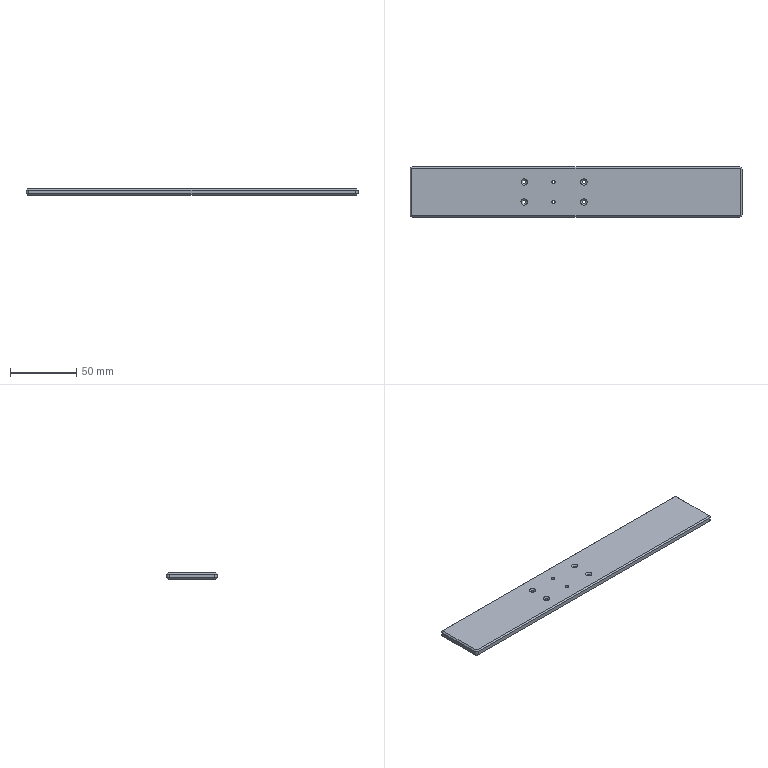Part | NX | 1 solid | 36 faces | box 250 x 38 x 5 mm | volume 46740 mm3 | plane 14 | cone 12 | cylinder 10 | commonest cylinder face diameters 2.459 x6 4 x4
STEP:
#1=CARTESIAN_POINT('',(6.,-5.071,0.));
#2=VERTEX_POINT('',#1);
#3=CARTESIAN_POINT('',(6.,-7.5,0.));
#4=DIRECTION('',(0.,0.,-1.));
#5=DIRECTION('',(0.,1.,0.));
#6=AXIS2_PLACEMENT_3D('',#3,#4,#5);
#7=CIRCLE('',#6,2.429);
#8=EDGE_CURVE('',#2,#2,#7,.T.);
#9=ORIENTED_EDGE('',*,*,#8,.F.);
#10=EDGE_LOOP('',(#9));
#11=FACE_BOUND('',#10,.T.);
#12=CARTESIAN_POINT('',(6.,-8.729,-1.2));
#13=VERTEX_POINT('',#12);
#14=CARTESIAN_POINT('',(6.,-7.5,-1.2));
#15=DIRECTION('',(0.,0.,1.));
#16=DIRECTION('',(0.,-1.,0.));
#17=AXIS2_PLACEMENT_3D('',#14,#15,#16);
#18=CIRCLE('',#17,1.23);
#19=EDGE_CURVE('',#13,#13,#18,.T.);
#20=ORIENTED_EDGE('',*,*,#19,.F.);
#21=EDGE_LOOP('',(#20));
#22=FACE_BOUND('',#21,.T.);
#23=CARTESIAN_POINT('',(6.,-7.5,-2.429));
#24=DIRECTION('',(0.,0.,1.));
#25=DIRECTION('',(-0.5,-0.866,0.));
#26=AXIS2_PLACEMENT_3D('',#23,#24,#25);
#27=CONICAL_SURFACE('',#26,0.,0.7854);
#28=ADVANCED_FACE('',(#11,#22),#27,.F.);
#29=CARTESIAN_POINT('',(-17.,6.271,0.));
#30=VERTEX_POINT('',#29);
#31=CARTESIAN_POINT('',(-17.,7.5,0.));
#32=DIRECTION('',(0.,0.,1.));
#33=DIRECTION('',(0.,-1.,0.));
#34=AXIS2_PLACEMENT_3D('',#31,#32,#33);
#35=CIRCLE('',#34,1.23);
#36=EDGE_CURVE('',#30,#30,#35,.T.);
#37=ORIENTED_EDGE('',*,*,#36,.F.);
#38=EDGE_LOOP('',(#37));
#39=FACE_BOUND('',#38,.T.);
#40=CARTESIAN_POINT('',(-17.,-8.729,0.));
#41=VERTEX_POINT('',#40);
#42=CARTESIAN_POINT('',(-17.,-7.5,0.));
#43=DIRECTION('',(0.,0.,1.));
#44=DIRECTION('',(0.,-1.,0.));
#45=AXIS2_PLACEMENT_3D('',#42,#43,#44);
#46=CIRCLE('',#45,1.23);
#47=EDGE_CURVE('',#41,#41,#46,.T.);
#48=ORIENTED_EDGE('',*,*,#47,.F.);
#49=EDGE_LOOP('',(#48));
#50=FACE_BOUND('',#49,.T.);
#51=CARTESIAN_POINT('',(-41.104,-6.285,0.));
#52=VERTEX_POINT('',#51);
#53=CARTESIAN_POINT('',(-39.,-7.5,0.));
#54=DIRECTION('',(0.,0.,-1.));
#55=DIRECTION('',(-0.866,0.5,0.));
#56=AXIS2_PLACEMENT_3D('',#53,#54,#55);
#57=CIRCLE('',#56,2.429);
#58=EDGE_CURVE('',#52,#52,#57,.T.);
#59=ORIENTED_EDGE('',*,*,#58,.T.);
#60=EDGE_LOOP('',(#59));
#61=FACE_BOUND('',#60,.T.);
#62=CARTESIAN_POINT('',(-39.,9.93,0.));
#63=VERTEX_POINT('',#62);
#64=CARTESIAN_POINT('',(-39.,7.5,0.));
#65=DIRECTION('',(0.,0.,-1.));
#66=DIRECTION('',(0.,1.,0.));
#67=AXIS2_PLACEMENT_3D('',#64,#65,#66);
#68=CIRCLE('',#67,2.429);
#69=EDGE_CURVE('',#63,#63,#68,.T.);
#70=ORIENTED_EDGE('',*,*,#69,.T.);
#71=EDGE_LOOP('',(#70));
#72=FACE_BOUND('',#71,.T.);
#73=CARTESIAN_POINT('',(6.,9.93,0.));
#74=VERTEX_POINT('',#73);
#75=CARTESIAN_POINT('',(6.,7.5,0.));
#76=DIRECTION('',(0.,0.,-1.));
#77=DIRECTION('',(0.,1.,0.));
#78=AXIS2_PLACEMENT_3D('',#75,#76,#77);
#79=CIRCLE('',#78,2.429);
#80=EDGE_CURVE('',#74,#74,#79,.T.);
#81=ORIENTED_EDGE('',*,*,#80,.T.);
#82=EDGE_LOOP('',(#81));
#83=FACE_BOUND('',#82,.T.);
#84=ORIENTED_EDGE('',*,*,#8,.T.);
#85=EDGE_LOOP('',(#84));
#86=FACE_BOUND('',#85,.T.);
#87=CARTESIAN_POINT('',(-123.,-18.,0.));
#88=VERTEX_POINT('',#87);
#89=CARTESIAN_POINT('',(-124.,-17.,0.));
#90=VERTEX_POINT('',#89);
#91=CARTESIAN_POINT('',(-123.,-17.,0.));
#92=DIRECTION('',(0.,0.,-1.));
#93=DIRECTION('',(-0.9659,-0.2588,0.));
#94=AXIS2_PLACEMENT_3D('',#91,#92,#93);
#95=CIRCLE('',#94,1.);
#96=EDGE_CURVE('',#88,#90,#95,.T.);
#97=ORIENTED_EDGE('',*,*,#96,.F.);
#98=CARTESIAN_POINT('',(123.,-18.,0.));
#99=VERTEX_POINT('',#98);
#100=CARTESIAN_POINT('',(0.,-18.,0.));
#101=DIRECTION('',(1.,0.,0.));
#102=VECTOR('',#101,1000.);
#103=LINE('',#100,#102);
#104=EDGE_CURVE('',#88,#99,#103,.T.);
#105=ORIENTED_EDGE('',*,*,#104,.T.);
#106=CARTESIAN_POINT('',(124.,-17.,0.));
#107=VERTEX_POINT('',#106);
#108=CARTESIAN_POINT('',(123.,-17.,0.));
#109=DIRECTION('',(0.,0.,-1.));
#110=DIRECTION('',(0.2588,-0.9659,0.));
#111=AXIS2_PLACEMENT_3D('',#108,#109,#110);
#112=CIRCLE('',#111,1.);
#113=EDGE_CURVE('',#107,#99,#112,.T.);
#114=ORIENTED_EDGE('',*,*,#113,.F.);
#115=CARTESIAN_POINT('',(124.,17.,0.));
#116=VERTEX_POINT('',#115);
#117=CARTESIAN_POINT('',(124.,0.,0.));
#118=DIRECTION('',(0.,1.,0.));
#119=VECTOR('',#118,1000.);
#120=LINE('',#117,#119);
#121=EDGE_CURVE('',#107,#116,#120,.T.);
#122=ORIENTED_EDGE('',*,*,#121,.T.);
#123=CARTESIAN_POINT('',(123.,18.,0.));
#124=VERTEX_POINT('',#123);
#125=CARTESIAN_POINT('',(123.,17.,0.));
#126=DIRECTION('',(0.,0.,-1.));
#127=DIRECTION('',(0.9659,0.2588,0.));
#128=AXIS2_PLACEMENT_3D('',#125,#126,#127);
#129=CIRCLE('',#128,1.);
#130=EDGE_CURVE('',#124,#116,#129,.T.);
#131=ORIENTED_EDGE('',*,*,#130,.F.);
#132=CARTESIAN_POINT('',(-123.,18.,0.));
#133=VERTEX_POINT('',#132);
#134=CARTESIAN_POINT('',(0.,18.,0.));
#135=DIRECTION('',(-1.,0.,0.));
#136=VECTOR('',#135,1000.);
#137=LINE('',#134,#136);
#138=EDGE_CURVE('',#124,#133,#137,.T.);
#139=ORIENTED_EDGE('',*,*,#138,.T.);
#140=CARTESIAN_POINT('',(-124.,17.,0.));
#141=VERTEX_POINT('',#140);
#142=CARTESIAN_POINT('',(-123.,17.,0.));
#143=DIRECTION('',(0.,0.,-1.));
#144=DIRECTION('',(-0.2588,0.9659,0.));
#145=AXIS2_PLACEMENT_3D('',#142,#143,#144);
#146=CIRCLE('',#145,1.);
#147=EDGE_CURVE('',#141,#133,#146,.T.);
#148=ORIENTED_EDGE('',*,*,#147,.F.);
#149=CARTESIAN_POINT('',(-124.,0.,0.));
#150=DIRECTION('',(0.,-1.,0.));
#151=VECTOR('',#150,1000.);
#152=LINE('',#149,#151);
#153=EDGE_CURVE('',#141,#90,#152,.T.);
#154=ORIENTED_EDGE('',*,*,#153,.T.);
#155=EDGE_LOOP('',(#97,#105,#114,#122,#131,#139,#148,#154));
#156=FACE_BOUND('',#155,.T.);
#157=CARTESIAN_POINT('',(0.,0.,0.));
#158=DIRECTION('',(0.,0.,-1.));
#159=DIRECTION('',(1.,0.,0.));
#160=AXIS2_PLACEMENT_3D('',#157,#158,#159);
#161=PLANE('',#160);
#162=ADVANCED_FACE('',(#39,#50,#61,#72,#83,#86,#156),#161,.F.);
#163=ORIENTED_EDGE('',*,*,#19,.T.);
#164=EDGE_LOOP('',(#163));
#165=FACE_BOUND('',#164,.T.);
#166=CARTESIAN_POINT('',(6.,-6.271,-5.));
#167=VERTEX_POINT('',#166);
#168=CARTESIAN_POINT('',(6.,-7.5,-5.));
#169=DIRECTION('',(0.,0.,-1.));
#170=DIRECTION('',(0.,1.,0.));
#171=AXIS2_PLACEMENT_3D('',#168,#169,#170);
#172=CIRCLE('',#171,1.23);
#173=EDGE_CURVE('',#167,#167,#172,.T.);
#174=ORIENTED_EDGE('',*,*,#173,.T.);
#175=EDGE_LOOP('',(#174));
#176=FACE_BOUND('',#175,.T.);
#177=CARTESIAN_POINT('',(6.,-7.5,-5.));
#178=DIRECTION('',(0.,0.,1.));
#179=DIRECTION('',(1.,0.,0.));
#180=AXIS2_PLACEMENT_3D('',#177,#178,#179);
#181=CYLINDRICAL_SURFACE('',#180,1.23);
#182=ADVANCED_FACE('',(#165,#176),#181,.F.);
#183=ORIENTED_EDGE('',*,*,#80,.F.);
#184=EDGE_LOOP('',(#183));
#185=FACE_BOUND('',#184,.T.);
#186=CARTESIAN_POINT('',(6.,6.271,-1.2));
#187=VERTEX_POINT('',#186);
#188=CARTESIAN_POINT('',(6.,7.5,-1.2));
#189=DIRECTION('',(0.,0.,1.));
#190=DIRECTION('',(0.,-1.,0.));
#191=AXIS2_PLACEMENT_3D('',#188,#189,#190);
#192=CIRCLE('',#191,1.23);
#193=EDGE_CURVE('',#187,#187,#192,.T.);
#194=ORIENTED_EDGE('',*,*,#193,.F.);
#195=EDGE_LOOP('',(#194));
#196=FACE_BOUND('',#195,.T.);
#197=CARTESIAN_POINT('',(6.,7.5,-2.429));
#198=DIRECTION('',(0.,0.,1.));
#199=DIRECTION('',(-0.5,-0.866,0.));
#200=AXIS2_PLACEMENT_3D('',#197,#198,#199);
#201=CONICAL_SURFACE('',#200,0.,0.7854);
#202=ADVANCED_FACE('',(#185,#196),#201,.F.);
#203=ORIENTED_EDGE('',*,*,#193,.T.);
#204=EDGE_LOOP('',(#203));
#205=FACE_BOUND('',#204,.T.);
#206=CARTESIAN_POINT('',(6.,8.729,-5.));
#207=VERTEX_POINT('',#206);
#208=CARTESIAN_POINT('',(6.,7.5,-5.));
#209=DIRECTION('',(0.,0.,-1.));
#210=DIRECTION('',(0.,1.,0.));
#211=AXIS2_PLACEMENT_3D('',#208,#209,#210);
#212=CIRCLE('',#211,1.23);
#213=EDGE_CURVE('',#207,#207,#212,.T.);
#214=ORIENTED_EDGE('',*,*,#213,.T.);
#215=EDGE_LOOP('',(#214));
#216=FACE_BOUND('',#215,.T.);
#217=CARTESIAN_POINT('',(6.,7.5,-5.));
#218=DIRECTION('',(0.,0.,1.));
#219=DIRECTION('',(1.,0.,0.));
#220=AXIS2_PLACEMENT_3D('',#217,#218,#219);
#221=CYLINDRICAL_SURFACE('',#220,1.23);
#222=ADVANCED_FACE('',(#205,#216),#221,.F.);
#223=ORIENTED_EDGE('',*,*,#69,.F.);
#224=EDGE_LOOP('',(#223));
#225=FACE_BOUND('',#224,.T.);
#226=CARTESIAN_POINT('',(-39.,6.271,-1.2));
#227=VERTEX_POINT('',#226);
#228=CARTESIAN_POINT('',(-39.,7.5,-1.2));
#229=DIRECTION('',(0.,0.,1.));
#230=DIRECTION('',(0.,-1.,0.));
#231=AXIS2_PLACEMENT_3D('',#228,#229,#230);
#232=CIRCLE('',#231,1.23);
#233=EDGE_CURVE('',#227,#227,#232,.T.);
#234=ORIENTED_EDGE('',*,*,#233,.F.);
#235=EDGE_LOOP('',(#234));
#236=FACE_BOUND('',#235,.T.);
#237=CARTESIAN_POINT('',(-39.,7.5,-2.429));
#238=DIRECTION('',(0.,0.,1.));
#239=DIRECTION('',(-0.5,-0.866,0.));
#240=AXIS2_PLACEMENT_3D('',#237,#238,#239);
#241=CONICAL_SURFACE('',#240,0.,0.7854);
#242=ADVANCED_FACE('',(#225,#236),#241,.F.);
#243=ORIENTED_EDGE('',*,*,#233,.T.);
#244=EDGE_LOOP('',(#243));
#245=FACE_BOUND('',#244,.T.);
#246=CARTESIAN_POINT('',(-39.,8.729,-5.));
#247=VERTEX_POINT('',#246);
#248=CARTESIAN_POINT('',(-39.,7.5,-5.));
#249=DIRECTION('',(0.,0.,-1.));
#250=DIRECTION('',(0.,1.,0.));
#251=AXIS2_PLACEMENT_3D('',#248,#249,#250);
#252=CIRCLE('',#251,1.23);
#253=EDGE_CURVE('',#247,#247,#252,.T.);
#254=ORIENTED_EDGE('',*,*,#253,.T.);
#255=EDGE_LOOP('',(#254));
#256=FACE_BOUND('',#255,.T.);
#257=CARTESIAN_POINT('',(-39.,7.5,-5.));
#258=DIRECTION('',(0.,0.,1.));
#259=DIRECTION('',(1.,0.,0.));
#260=AXIS2_PLACEMENT_3D('',#257,#258,#259);
#261=CYLINDRICAL_SURFACE('',#260,1.23);
#262=ADVANCED_FACE('',(#245,#256),#261,.F.);
#263=ORIENTED_EDGE('',*,*,#58,.F.);
#264=EDGE_LOOP('',(#263));
#265=FACE_BOUND('',#264,.T.);
#266=CARTESIAN_POINT('',(-39.,-8.729,-1.2));
#267=VERTEX_POINT('',#266);
#268=CARTESIAN_POINT('',(-39.,-7.5,-1.2));
#269=DIRECTION('',(0.,0.,1.));
#270=DIRECTION('',(0.,-1.,0.));
#271=AXIS2_PLACEMENT_3D('',#268,#269,#270);
#272=CIRCLE('',#271,1.23);
#273=EDGE_CURVE('',#267,#267,#272,.T.);
#274=ORIENTED_EDGE('',*,*,#273,.F.);
#275=EDGE_LOOP('',(#274));
#276=FACE_BOUND('',#275,.T.);
#277=CARTESIAN_POINT('',(-39.,-7.5,-2.429));
#278=DIRECTION('',(0.,0.,1.));
#279=DIRECTION('',(-0.5,-0.866,0.));
#280=AXIS2_PLACEMENT_3D('',#277,#278,#279);
#281=CONICAL_SURFACE('',#280,0.,0.7854);
#282=ADVANCED_FACE('',(#265,#276),#281,.F.);
#283=ORIENTED_EDGE('',*,*,#273,.T.);
#284=EDGE_LOOP('',(#283));
#285=FACE_BOUND('',#284,.T.);
#286=CARTESIAN_POINT('',(-39.,-6.271,-5.));
#287=VERTEX_POINT('',#286);
#288=CARTESIAN_POINT('',(-39.,-7.5,-5.));
#289=DIRECTION('',(0.,0.,-1.));
#290=DIRECTION('',(0.,1.,0.));
#291=AXIS2_PLACEMENT_3D('',#288,#289,#290);
#292=CIRCLE('',#291,1.23);
#293=EDGE_CURVE('',#287,#287,#292,.T.);
#294=ORIENTED_EDGE('',*,*,#293,.T.);
#295=EDGE_LOOP('',(#294));
#296=FACE_BOUND('',#295,.T.);
#297=CARTESIAN_POINT('',(-39.,-7.5,-5.));
#298=DIRECTION('',(0.,0.,1.));
#299=DIRECTION('',(1.,0.,0.));
#300=AXIS2_PLACEMENT_3D('',#297,#298,#299);
#301=CYLINDRICAL_SURFACE('',#300,1.23);
#302=ADVANCED_FACE('',(#285,#296),#301,.F.);
#303=CARTESIAN_POINT('',(-123.,-19.,-1.));
#304=VERTEX_POINT('',#303);
#305=CARTESIAN_POINT('',(-123.,-18.5,-0.5));
#306=DIRECTION('',(0.,-0.7071,-0.7071));
#307=VECTOR('',#306,1000.);
#308=LINE('',#305,#307);
#309=EDGE_CURVE('',#88,#304,#308,.T.);
#310=ORIENTED_EDGE('',*,*,#309,.F.);
#311=ORIENTED_EDGE('',*,*,#96,.T.);
#312=CARTESIAN_POINT('',(-125.,-17.,-1.));
#313=VERTEX_POINT('',#312);
#314=CARTESIAN_POINT('',(-124.5,-17.,-0.5));
#315=DIRECTION('',(-0.7071,0.,-0.7071));
#316=VECTOR('',#315,1000.);
#317=LINE('',#314,#316);
#318=EDGE_CURVE('',#90,#313,#317,.T.);
#319=ORIENTED_EDGE('',*,*,#318,.T.);
#320=CARTESIAN_POINT('',(-123.,-17.,-1.));
#321=DIRECTION('',(0.,0.,-1.));
#322=DIRECTION('',(0.,1.,0.));
#323=AXIS2_PLACEMENT_3D('',#320,#321,#322);
#324=CIRCLE('',#323,2.);
#325=EDGE_CURVE('',#304,#313,#324,.T.);
#326=ORIENTED_EDGE('',*,*,#325,.F.);
#327=EDGE_LOOP('',(#310,#311,#319,#326));
#328=FACE_BOUND('',#327,.T.);
#329=CARTESIAN_POINT('',(-123.,-17.,1.));
#330=DIRECTION('',(0.,0.,-1.));
#331=DIRECTION('',(0.2588,-0.9659,0.));
#332=AXIS2_PLACEMENT_3D('',#329,#330,#331);
#333=CONICAL_SURFACE('',#332,0.,0.7854);
#334=ADVANCED_FACE('',(#328),#333,.T.);
#335=CARTESIAN_POINT('',(123.,-19.,-1.));
#336=VERTEX_POINT('',#335);
#337=CARTESIAN_POINT('',(123.,-18.5,-0.5));
#338=DIRECTION('',(0.,-0.7071,-0.7071));
#339=VECTOR('',#338,1000.);
#340=LINE('',#337,#339);
#341=EDGE_CURVE('',#99,#336,#340,.T.);
#342=ORIENTED_EDGE('',*,*,#341,.F.);
#343=ORIENTED_EDGE('',*,*,#104,.F.);
#344=ORIENTED_EDGE('',*,*,#309,.T.);
#345=CARTESIAN_POINT('',(0.,-19.,-1.));
#346=DIRECTION('',(1.,0.,0.));
#347=VECTOR('',#346,1000.);
#348=LINE('',#345,#347);
#349=EDGE_CURVE('',#304,#336,#348,.T.);
#350=ORIENTED_EDGE('',*,*,#349,.T.);
#351=EDGE_LOOP('',(#342,#343,#344,#350));
#352=FACE_BOUND('',#351,.T.);
#353=CARTESIAN_POINT('',(0.,-18.,0.));
#354=DIRECTION('',(0.,0.7071,-0.7071));
#355=DIRECTION('',(1.,0.,0.));
#356=AXIS2_PLACEMENT_3D('',#353,#354,#355);
#357=PLANE('',#356);
#358=ADVANCED_FACE('',(#352),#357,.F.);
#359=CARTESIAN_POINT('',(125.,-17.,-1.));
#360=VERTEX_POINT('',#359);
#361=CARTESIAN_POINT('',(124.5,-17.,-0.5));
#362=DIRECTION('',(0.7071,0.,-0.7071));
#363=VECTOR('',#362,1000.);
#364=LINE('',#361,#363);
#365=EDGE_CURVE('',#107,#360,#364,.T.);
#366=ORIENTED_EDGE('',*,*,#365,.F.);
#367=ORIENTED_EDGE('',*,*,#113,.T.);
#368=ORIENTED_EDGE('',*,*,#341,.T.);
#369=CARTESIAN_POINT('',(123.,-17.,-1.));
#370=DIRECTION('',(0.,0.,-1.));
#371=DIRECTION('',(0.,1.,0.));
#372=AXIS2_PLACEMENT_3D('',#369,#370,#371);
#373=CIRCLE('',#372,2.);
#374=EDGE_CURVE('',#360,#336,#373,.T.);
#375=ORIENTED_EDGE('',*,*,#374,.F.);
#376=EDGE_LOOP('',(#366,#367,#368,#375));
#377=FACE_BOUND('',#376,.T.);
#378=CARTESIAN_POINT('',(123.,-17.,1.));
#379=DIRECTION('',(0.,0.,-1.));
#380=DIRECTION('',(0.9659,0.2588,0.));
#381=AXIS2_PLACEMENT_3D('',#378,#379,#380);
#382=CONICAL_SURFACE('',#381,0.,0.7854);
#383=ADVANCED_FACE('',(#377),#382,.T.);
#384=CARTESIAN_POINT('',(125.,17.,-1.));
#385=VERTEX_POINT('',#384);
#386=CARTESIAN_POINT('',(124.5,17.,-0.5));
#387=DIRECTION('',(0.7071,0.,-0.7071));
#388=VECTOR('',#387,1000.);
#389=LINE('',#386,#388);
#390=EDGE_CURVE('',#116,#385,#389,.T.);
#391=ORIENTED_EDGE('',*,*,#390,.F.);
#392=ORIENTED_EDGE('',*,*,#121,.F.);
#393=ORIENTED_EDGE('',*,*,#365,.T.);
#394=CARTESIAN_POINT('',(125.,0.,-1.));
#395=DIRECTION('',(0.,1.,0.));
#396=VECTOR('',#395,1000.);
#397=LINE('',#394,#396);
#398=EDGE_CURVE('',#360,#385,#397,.T.);
#399=ORIENTED_EDGE('',*,*,#398,.T.);
#400=EDGE_LOOP('',(#391,#392,#393,#399));
#401=FACE_BOUND('',#400,.T.);
#402=CARTESIAN_POINT('',(124.,0.,0.));
#403=DIRECTION('',(-0.7071,0.,-0.7071));
#404=DIRECTION('',(0.,1.,0.));
#405=AXIS2_PLACEMENT_3D('',#402,#403,#404);
#406=PLANE('',#405);
#407=ADVANCED_FACE('',(#401),#406,.F.);
#408=CARTESIAN_POINT('',(123.,19.,-1.));
#409=VERTEX_POINT('',#408);
#410=CARTESIAN_POINT('',(123.,18.5,-0.5));
#411=DIRECTION('',(0.,0.7071,-0.7071));
#412=VECTOR('',#411,1000.);
#413=LINE('',#410,#412);
#414=EDGE_CURVE('',#124,#409,#413,.T.);
#415=ORIENTED_EDGE('',*,*,#414,.F.);
#416=ORIENTED_EDGE('',*,*,#130,.T.);
#417=ORIENTED_EDGE('',*,*,#390,.T.);
#418=CARTESIAN_POINT('',(123.,17.,-1.));
#419=DIRECTION('',(0.,0.,-1.));
#420=DIRECTION('',(0.,1.,0.));
#421=AXIS2_PLACEMENT_3D('',#418,#419,#420);
#422=CIRCLE('',#421,2.);
#423=EDGE_CURVE('',#409,#385,#422,.T.);
#424=ORIENTED_EDGE('',*,*,#423,.F.);
#425=EDGE_LOOP('',(#415,#416,#417,#424));
#426=FACE_BOUND('',#425,.T.);
#427=CARTESIAN_POINT('',(123.,17.,1.));
#428=DIRECTION('',(0.,0.,-1.));
#429=DIRECTION('',(-0.2588,0.9659,0.));
#430=AXIS2_PLACEMENT_3D('',#427,#428,#429);
#431=CONICAL_SURFACE('',#430,0.,0.7854);
#432=ADVANCED_FACE('',(#426),#431,.T.);
#433=CARTESIAN_POINT('',(-123.,19.,-1.));
#434=VERTEX_POINT('',#433);
#435=CARTESIAN_POINT('',(-123.,18.5,-0.5));
#436=DIRECTION('',(0.,0.7071,-0.7071));
#437=VECTOR('',#436,1000.);
#438=LINE('',#435,#437);
#439=EDGE_CURVE('',#133,#434,#438,.T.);
#440=ORIENTED_EDGE('',*,*,#439,.F.);
#441=ORIENTED_EDGE('',*,*,#138,.F.);
#442=ORIENTED_EDGE('',*,*,#414,.T.);
#443=CARTESIAN_POINT('',(0.,19.,-1.));
#444=DIRECTION('',(-1.,0.,0.));
#445=VECTOR('',#444,1000.);
#446=LINE('',#443,#445);
#447=EDGE_CURVE('',#409,#434,#446,.T.);
#448=ORIENTED_EDGE('',*,*,#447,.T.);
#449=EDGE_LOOP('',(#440,#441,#442,#448));
#450=FACE_BOUND('',#449,.T.);
#451=CARTESIAN_POINT('',(0.,18.,0.));
#452=DIRECTION('',(0.,-0.7071,-0.7071));
#453=DIRECTION('',(-1.,0.,0.));
#454=AXIS2_PLACEMENT_3D('',#451,#452,#453);
#455=PLANE('',#454);
#456=ADVANCED_FACE('',(#450),#455,.F.);
#457=CARTESIAN_POINT('',(-125.,17.,-1.));
#458=VERTEX_POINT('',#457);
#459=CARTESIAN_POINT('',(-124.5,17.,-0.5));
#460=DIRECTION('',(-0.7071,0.,-0.7071));
#461=VECTOR('',#460,1000.);
#462=LINE('',#459,#461);
#463=EDGE_CURVE('',#141,#458,#462,.T.);
#464=ORIENTED_EDGE('',*,*,#463,.F.);
#465=ORIENTED_EDGE('',*,*,#147,.T.);
#466=ORIENTED_EDGE('',*,*,#439,.T.);
#467=CARTESIAN_POINT('',(-123.,17.,-1.));
#468=DIRECTION('',(0.,0.,-1.));
#469=DIRECTION('',(0.,1.,0.));
#470=AXIS2_PLACEMENT_3D('',#467,#468,#469);
#471=CIRCLE('',#470,2.);
#472=EDGE_CURVE('',#458,#434,#471,.T.);
#473=ORIENTED_EDGE('',*,*,#472,.F.);
#474=EDGE_LOOP('',(#464,#465,#466,#473));
#475=FACE_BOUND('',#474,.T.);
#476=CARTESIAN_POINT('',(-123.,17.,1.));
#477=DIRECTION('',(0.,0.,-1.));
#478=DIRECTION('',(-0.9659,-0.2588,0.));
#479=AXIS2_PLACEMENT_3D('',#476,#477,#478);
#480=CONICAL_SURFACE('',#479,0.,0.7854);
#481=ADVANCED_FACE('',(#475),#480,.T.);
#482=ORIENTED_EDGE('',*,*,#318,.F.);
#483=ORIENTED_EDGE('',*,*,#153,.F.);
#484=ORIENTED_EDGE('',*,*,#463,.T.);
#485=CARTESIAN_POINT('',(-125.,0.,-1.));
#486=DIRECTION('',(0.,-1.,0.));
#487=VECTOR('',#486,1000.);
#488=LINE('',#485,#487);
#489=EDGE_CURVE('',#458,#313,#488,.T.);
#490=ORIENTED_EDGE('',*,*,#489,.T.);
#491=EDGE_LOOP('',(#482,#483,#484,#490));
#492=FACE_BOUND('',#491,.T.);
#493=CARTESIAN_POINT('',(-124.,0.,0.));
#494=DIRECTION('',(0.7071,0.,-0.7071));
#495=DIRECTION('',(0.,-1.,0.));
#496=AXIS2_PLACEMENT_3D('',#493,#494,#495);
#497=PLANE('',#496);
#498=ADVANCED_FACE('',(#492),#497,.F.);
#499=ORIENTED_EDGE('',*,*,#398,.F.);
#500=CARTESIAN_POINT('',(125.,-17.,-4.));
#501=VERTEX_POINT('',#500);
#502=CARTESIAN_POINT('',(125.,-17.,-2.5));
#503=DIRECTION('',(0.,0.,-1.));
#504=VECTOR('',#503,1000.);
#505=LINE('',#502,#504);
#506=EDGE_CURVE('',#360,#501,#505,.T.);
#507=ORIENTED_EDGE('',*,*,#506,.T.);
#508=CARTESIAN_POINT('',(125.,17.,-4.));
#509=VERTEX_POINT('',#508);
#510=CARTESIAN_POINT('',(125.,0.,-4.));
#511=DIRECTION('',(0.,1.,0.));
#512=VECTOR('',#511,1000.);
#513=LINE('',#510,#512);
#514=EDGE_CURVE('',#501,#509,#513,.T.);
#515=ORIENTED_EDGE('',*,*,#514,.T.);
#516=CARTESIAN_POINT('',(125.,17.,-2.5));
#517=DIRECTION('',(0.,0.,-1.));
#518=VECTOR('',#517,1000.);
#519=LINE('',#516,#518);
#520=EDGE_CURVE('',#385,#509,#519,.T.);
#521=ORIENTED_EDGE('',*,*,#520,.F.);
#522=EDGE_LOOP('',(#499,#507,#515,#521));
#523=FACE_BOUND('',#522,.T.);
#524=CARTESIAN_POINT('',(125.,-19.,0.));
#525=DIRECTION('',(-1.,0.,0.));
#526=DIRECTION('',(0.,1.,0.));
#527=AXIS2_PLACEMENT_3D('',#524,#525,#526);
#528=PLANE('',#527);
#529=ADVANCED_FACE('',(#523),#528,.F.);
#530=ORIENTED_EDGE('',*,*,#520,.T.);
#531=CARTESIAN_POINT('',(123.,19.,-4.));
#532=VERTEX_POINT('',#531);
#533=CARTESIAN_POINT('',(123.,17.,-4.));
#534=DIRECTION('',(0.,0.,-1.));
#535=DIRECTION('',(-0.9659,-0.2588,0.));
#536=AXIS2_PLACEMENT_3D('',#533,#534,#535);
#537=CIRCLE('',#536,2.);
#538=EDGE_CURVE('',#532,#509,#537,.T.);
#539=ORIENTED_EDGE('',*,*,#538,.F.);
#540=CARTESIAN_POINT('',(123.,19.,-2.5));
#541=DIRECTION('',(0.,0.,-1.));
#542=VECTOR('',#541,1000.);
#543=LINE('',#540,#542);
#544=EDGE_CURVE('',#409,#532,#543,.T.);
#545=ORIENTED_EDGE('',*,*,#544,.F.);
#546=ORIENTED_EDGE('',*,*,#423,.T.);
#547=EDGE_LOOP('',(#530,#539,#545,#546));
#548=FACE_BOUND('',#547,.T.);
#549=CARTESIAN_POINT('',(123.,17.,-2.5));
#550=DIRECTION('',(0.,0.,-1.));
#551=DIRECTION('',(0.,1.,0.));
#552=AXIS2_PLACEMENT_3D('',#549,#550,#551);
#553=CYLINDRICAL_SURFACE('',#552,2.);
#554=ADVANCED_FACE('',(#548),#553,.T.);
#555=ORIENTED_EDGE('',*,*,#447,.F.);
#556=ORIENTED_EDGE('',*,*,#544,.T.);
#557=CARTESIAN_POINT('',(-123.,19.,-4.));
#558=VERTEX_POINT('',#557);
#559=CARTESIAN_POINT('',(0.,19.,-4.));
#560=DIRECTION('',(-1.,0.,0.));
#561=VECTOR('',#560,1000.);
#562=LINE('',#559,#561);
#563=EDGE_CURVE('',#532,#558,#562,.T.);
#564=ORIENTED_EDGE('',*,*,#563,.T.);
#565=CARTESIAN_POINT('',(-123.,19.,-2.5));
#566=DIRECTION('',(0.,0.,-1.));
#567=VECTOR('',#566,1000.);
#568=LINE('',#565,#567);
#569=EDGE_CURVE('',#434,#558,#568,.T.);
#570=ORIENTED_EDGE('',*,*,#569,.F.);
#571=EDGE_LOOP('',(#555,#556,#564,#570));
#572=FACE_BOUND('',#571,.T.);
#573=CARTESIAN_POINT('',(125.,19.,0.));
#574=DIRECTION('',(0.,-1.,0.));
#575=DIRECTION('',(-1.,0.,0.));
#576=AXIS2_PLACEMENT_3D('',#573,#574,#575);
#577=PLANE('',#576);
#578=ADVANCED_FACE('',(#572),#577,.F.);
#579=ORIENTED_EDGE('',*,*,#569,.T.);
#580=CARTESIAN_POINT('',(-125.,17.,-4.));
#581=VERTEX_POINT('',#580);
#582=CARTESIAN_POINT('',(-123.,17.,-4.));
#583=DIRECTION('',(0.,0.,-1.));
#584=DIRECTION('',(0.2588,-0.9659,0.));
#585=AXIS2_PLACEMENT_3D('',#582,#583,#584);
#586=CIRCLE('',#585,2.);
#587=EDGE_CURVE('',#581,#558,#586,.T.);
#588=ORIENTED_EDGE('',*,*,#587,.F.);
#589=CARTESIAN_POINT('',(-125.,17.,-2.5));
#590=DIRECTION('',(0.,0.,-1.));
#591=VECTOR('',#590,1000.);
#592=LINE('',#589,#591);
#593=EDGE_CURVE('',#458,#581,#592,.T.);
#594=ORIENTED_EDGE('',*,*,#593,.F.);
#595=ORIENTED_EDGE('',*,*,#472,.T.);
#596=EDGE_LOOP('',(#579,#588,#594,#595));
#597=FACE_BOUND('',#596,.T.);
#598=CARTESIAN_POINT('',(-123.,17.,-2.5));
#599=DIRECTION('',(0.,0.,-1.));
#600=DIRECTION('',(-1.,0.,0.));
#601=AXIS2_PLACEMENT_3D('',#598,#599,#600);
#602=CYLINDRICAL_SURFACE('',#601,2.);
#603=ADVANCED_FACE('',(#597),#602,.T.);
#604=ORIENTED_EDGE('',*,*,#489,.F.);
#605=ORIENTED_EDGE('',*,*,#593,.T.);
#606=CARTESIAN_POINT('',(-125.,-17.,-4.));
#607=VERTEX_POINT('',#606);
#608=CARTESIAN_POINT('',(-125.,0.,-4.));
#609=DIRECTION('',(0.,-1.,0.));
#610=VECTOR('',#609,1000.);
#611=LINE('',#608,#610);
#612=EDGE_CURVE('',#581,#607,#611,.T.);
#613=ORIENTED_EDGE('',*,*,#612,.T.);
#614=CARTESIAN_POINT('',(-125.,-17.,-2.5));
#615=DIRECTION('',(0.,0.,-1.));
#616=VECTOR('',#615,1000.);
#617=LINE('',#614,#616);
#618=EDGE_CURVE('',#313,#607,#617,.T.);
#619=ORIENTED_EDGE('',*,*,#618,.F.);
#620=EDGE_LOOP('',(#604,#605,#613,#619));
#621=FACE_BOUND('',#620,.T.);
#622=CARTESIAN_POINT('',(-125.,19.,0.));
#623=DIRECTION('',(1.,0.,0.));
#624=DIRECTION('',(0.,-1.,0.));
#625=AXIS2_PLACEMENT_3D('',#622,#623,#624);
#626=PLANE('',#625);
#627=ADVANCED_FACE('',(#621),#626,.F.);
#628=CARTESIAN_POINT('',(123.,-19.,-4.));
#629=VERTEX_POINT('',#628);
#630=CARTESIAN_POINT('',(123.,-19.,-2.5));
#631=DIRECTION('',(0.,0.,-1.));
#632=VECTOR('',#631,1000.);
#633=LINE('',#630,#632);
#634=EDGE_CURVE('',#336,#629,#633,.T.);
#635=ORIENTED_EDGE('',*,*,#634,.T.);
#636=CARTESIAN_POINT('',(123.,-17.,-4.));
#637=DIRECTION('',(0.,0.,-1.));
#638=DIRECTION('',(-0.2588,0.9659,0.));
#639=AXIS2_PLACEMENT_3D('',#636,#637,#638);
#640=CIRCLE('',#639,2.);
#641=EDGE_CURVE('',#501,#629,#640,.T.);
#642=ORIENTED_EDGE('',*,*,#641,.F.);
#643=ORIENTED_EDGE('',*,*,#506,.F.);
#644=ORIENTED_EDGE('',*,*,#374,.T.);
#645=EDGE_LOOP('',(#635,#642,#643,#644));
#646=FACE_BOUND('',#645,.T.);
#647=CARTESIAN_POINT('',(123.,-17.,-2.5));
#648=DIRECTION('',(0.,0.,-1.));
#649=DIRECTION('',(1.,0.,0.));
#650=AXIS2_PLACEMENT_3D('',#647,#648,#649);
#651=CYLINDRICAL_SURFACE('',#650,2.);
#652=ADVANCED_FACE('',(#646),#651,.T.);
#653=ORIENTED_EDGE('',*,*,#618,.T.);
#654=CARTESIAN_POINT('',(-123.,-19.,-4.));
#655=VERTEX_POINT('',#654);
#656=CARTESIAN_POINT('',(-123.,-17.,-4.));
#657=DIRECTION('',(0.,0.,-1.));
#658=DIRECTION('',(0.9659,0.2588,0.));
#659=AXIS2_PLACEMENT_3D('',#656,#657,#658);
#660=CIRCLE('',#659,2.);
#661=EDGE_CURVE('',#655,#607,#660,.T.);
#662=ORIENTED_EDGE('',*,*,#661,.F.);
#663=CARTESIAN_POINT('',(-123.,-19.,-2.5));
#664=DIRECTION('',(0.,0.,-1.));
#665=VECTOR('',#664,1000.);
#666=LINE('',#663,#665);
#667=EDGE_CURVE('',#304,#655,#666,.T.);
#668=ORIENTED_EDGE('',*,*,#667,.F.);
#669=ORIENTED_EDGE('',*,*,#325,.T.);
#670=EDGE_LOOP('',(#653,#662,#668,#669));
#671=FACE_BOUND('',#670,.T.);
#672=CARTESIAN_POINT('',(-123.,-17.,-2.5));
#673=DIRECTION('',(0.,0.,-1.));
#674=DIRECTION('',(0.,-1.,0.));
#675=AXIS2_PLACEMENT_3D('',#672,#673,#674);
#676=CYLINDRICAL_SURFACE('',#675,2.);
#677=ADVANCED_FACE('',(#671),#676,.T.);
#678=ORIENTED_EDGE('',*,*,#349,.F.);
#679=ORIENTED_EDGE('',*,*,#667,.T.);
#680=CARTESIAN_POINT('',(0.,-19.,-4.));
#681=DIRECTION('',(1.,0.,0.));
#682=VECTOR('',#681,1000.);
#683=LINE('',#680,#682);
#684=EDGE_CURVE('',#655,#629,#683,.T.);
#685=ORIENTED_EDGE('',*,*,#684,.T.);
#686=ORIENTED_EDGE('',*,*,#634,.F.);
#687=EDGE_LOOP('',(#678,#679,#685,#686));
#688=FACE_BOUND('',#687,.T.);
#689=CARTESIAN_POINT('',(-125.,-19.,0.));
#690=DIRECTION('',(0.,1.,0.));
#691=DIRECTION('',(1.,0.,0.));
#692=AXIS2_PLACEMENT_3D('',#689,#690,#691);
#693=PLANE('',#692);
#694=ADVANCED_FACE('',(#688),#693,.F.);
#695=CARTESIAN_POINT('',(124.,-17.,-5.));
#696=VERTEX_POINT('',#695);
#697=CARTESIAN_POINT('',(124.5,-17.,-4.5));
#698=DIRECTION('',(-0.7071,0.,-0.7071));
#699=VECTOR('',#698,1000.);
#700=LINE('',#697,#699);
#701=EDGE_CURVE('',#501,#696,#700,.T.);
#702=ORIENTED_EDGE('',*,*,#701,.F.);
#703=ORIENTED_EDGE('',*,*,#641,.T.);
#704=CARTESIAN_POINT('',(123.,-18.,-5.));
#705=VERTEX_POINT('',#704);
#706=CARTESIAN_POINT('',(123.,-18.5,-4.5));
#707=DIRECTION('',(0.,0.7071,-0.7071));
#708=VECTOR('',#707,1000.);
#709=LINE('',#706,#708);
#710=EDGE_CURVE('',#629,#705,#709,.T.);
#711=ORIENTED_EDGE('',*,*,#710,.T.);
#712=CARTESIAN_POINT('',(123.,-17.,-5.));
#713=DIRECTION('',(0.,0.,-1.));
#714=DIRECTION('',(0.,1.,0.));
#715=AXIS2_PLACEMENT_3D('',#712,#713,#714);
#716=CIRCLE('',#715,1.);
#717=EDGE_CURVE('',#696,#705,#716,.T.);
#718=ORIENTED_EDGE('',*,*,#717,.F.);
#719=EDGE_LOOP('',(#702,#703,#711,#718));
#720=FACE_BOUND('',#719,.T.);
#721=CARTESIAN_POINT('',(123.,-17.,-6.));
#722=DIRECTION('',(0.,0.,1.));
#723=DIRECTION('',(0.9659,0.2588,0.));
#724=AXIS2_PLACEMENT_3D('',#721,#722,#723);
#725=CONICAL_SURFACE('',#724,0.,0.7854);
#726=ADVANCED_FACE('',(#720),#725,.T.);
#727=CARTESIAN_POINT('',(124.,17.,-5.));
#728=VERTEX_POINT('',#727);
#729=CARTESIAN_POINT('',(124.5,17.,-4.5));
#730=DIRECTION('',(0.7071,0.,0.7071));
#731=VECTOR('',#730,1000.);
#732=LINE('',#729,#731);
#733=EDGE_CURVE('',#728,#509,#732,.T.);
#734=ORIENTED_EDGE('',*,*,#733,.T.);
#735=ORIENTED_EDGE('',*,*,#514,.F.);
#736=ORIENTED_EDGE('',*,*,#701,.T.);
#737=CARTESIAN_POINT('',(124.,0.,-5.));
#738=DIRECTION('',(0.,1.,0.));
#739=VECTOR('',#738,1000.);
#740=LINE('',#737,#739);
#741=EDGE_CURVE('',#696,#728,#740,.T.);
#742=ORIENTED_EDGE('',*,*,#741,.T.);
#743=EDGE_LOOP('',(#734,#735,#736,#742));
#744=FACE_BOUND('',#743,.T.);
#745=CARTESIAN_POINT('',(125.,0.,-4.));
#746=DIRECTION('',(-0.7071,0.,0.7071));
#747=DIRECTION('',(0.,1.,0.));
#748=AXIS2_PLACEMENT_3D('',#745,#746,#747);
#749=PLANE('',#748);
#750=ADVANCED_FACE('',(#744),#749,.F.);
#751=CARTESIAN_POINT('',(123.,18.,-5.));
#752=VERTEX_POINT('',#751);
#753=CARTESIAN_POINT('',(123.,18.5,-4.5));
#754=DIRECTION('',(0.,-0.7071,-0.7071));
#755=VECTOR('',#754,1000.);
#756=LINE('',#753,#755);
#757=EDGE_CURVE('',#532,#752,#756,.T.);
#758=ORIENTED_EDGE('',*,*,#757,.F.);
#759=ORIENTED_EDGE('',*,*,#538,.T.);
#760=ORIENTED_EDGE('',*,*,#733,.F.);
#761=CARTESIAN_POINT('',(123.,17.,-5.));
#762=DIRECTION('',(0.,0.,-1.));
#763=DIRECTION('',(0.,1.,0.));
#764=AXIS2_PLACEMENT_3D('',#761,#762,#763);
#765=CIRCLE('',#764,1.);
#766=EDGE_CURVE('',#752,#728,#765,.T.);
#767=ORIENTED_EDGE('',*,*,#766,.F.);
#768=EDGE_LOOP('',(#758,#759,#760,#767));
#769=FACE_BOUND('',#768,.T.);
#770=CARTESIAN_POINT('',(123.,17.,-6.));
#771=DIRECTION('',(0.,0.,1.));
#772=DIRECTION('',(-0.2588,0.9659,0.));
#773=AXIS2_PLACEMENT_3D('',#770,#771,#772);
#774=CONICAL_SURFACE('',#773,0.,0.7854);
#775=ADVANCED_FACE('',(#769),#774,.T.);
#776=CARTESIAN_POINT('',(-123.,18.,-5.));
#777=VERTEX_POINT('',#776);
#778=CARTESIAN_POINT('',(-123.,18.5,-4.5));
#779=DIRECTION('',(0.,0.7071,0.7071));
#780=VECTOR('',#779,1000.);
#781=LINE('',#778,#780);
#782=EDGE_CURVE('',#777,#558,#781,.T.);
#783=ORIENTED_EDGE('',*,*,#782,.T.);
#784=ORIENTED_EDGE('',*,*,#563,.F.);
#785=ORIENTED_EDGE('',*,*,#757,.T.);
#786=CARTESIAN_POINT('',(0.,18.,-5.));
#787=DIRECTION('',(-1.,0.,0.));
#788=VECTOR('',#787,1000.);
#789=LINE('',#786,#788);
#790=EDGE_CURVE('',#752,#777,#789,.T.);
#791=ORIENTED_EDGE('',*,*,#790,.T.);
#792=EDGE_LOOP('',(#783,#784,#785,#791));
#793=FACE_BOUND('',#792,.T.);
#794=CARTESIAN_POINT('',(0.,19.,-4.));
#795=DIRECTION('',(0.,-0.7071,0.7071));
#796=DIRECTION('',(-1.,0.,0.));
#797=AXIS2_PLACEMENT_3D('',#794,#795,#796);
#798=PLANE('',#797);
#799=ADVANCED_FACE('',(#793),#798,.F.);
#800=CARTESIAN_POINT('',(-124.,17.,-5.));
#801=VERTEX_POINT('',#800);
#802=CARTESIAN_POINT('',(-124.5,17.,-4.5));
#803=DIRECTION('',(0.7071,0.,-0.7071));
#804=VECTOR('',#803,1000.);
#805=LINE('',#802,#804);
#806=EDGE_CURVE('',#581,#801,#805,.T.);
#807=ORIENTED_EDGE('',*,*,#806,.F.);
#808=ORIENTED_EDGE('',*,*,#587,.T.);
#809=ORIENTED_EDGE('',*,*,#782,.F.);
#810=CARTESIAN_POINT('',(-123.,17.,-5.));
#811=DIRECTION('',(0.,0.,-1.));
#812=DIRECTION('',(0.,1.,0.));
#813=AXIS2_PLACEMENT_3D('',#810,#811,#812);
#814=CIRCLE('',#813,1.);
#815=EDGE_CURVE('',#801,#777,#814,.T.);
#816=ORIENTED_EDGE('',*,*,#815,.F.);
#817=EDGE_LOOP('',(#807,#808,#809,#816));
#818=FACE_BOUND('',#817,.T.);
#819=CARTESIAN_POINT('',(-123.,17.,-6.));
#820=DIRECTION('',(0.,0.,1.));
#821=DIRECTION('',(-0.9659,-0.2588,0.));
#822=AXIS2_PLACEMENT_3D('',#819,#820,#821);
#823=CONICAL_SURFACE('',#822,0.,0.7854);
#824=ADVANCED_FACE('',(#818),#823,.T.);
#825=CARTESIAN_POINT('',(-124.,-17.,-5.));
#826=VERTEX_POINT('',#825);
#827=CARTESIAN_POINT('',(-124.5,-17.,-4.5));
#828=DIRECTION('',(-0.7071,0.,0.7071));
#829=VECTOR('',#828,1000.);
#830=LINE('',#827,#829);
#831=EDGE_CURVE('',#826,#607,#830,.T.);
#832=ORIENTED_EDGE('',*,*,#831,.T.);
#833=ORIENTED_EDGE('',*,*,#612,.F.);
#834=ORIENTED_EDGE('',*,*,#806,.T.);
#835=CARTESIAN_POINT('',(-124.,0.,-5.));
#836=DIRECTION('',(0.,-1.,0.));
#837=VECTOR('',#836,1000.);
#838=LINE('',#835,#837);
#839=EDGE_CURVE('',#801,#826,#838,.T.);
#840=ORIENTED_EDGE('',*,*,#839,.T.);
#841=EDGE_LOOP('',(#832,#833,#834,#840));
#842=FACE_BOUND('',#841,.T.);
#843=CARTESIAN_POINT('',(-125.,0.,-4.));
#844=DIRECTION('',(0.7071,0.,0.7071));
#845=DIRECTION('',(0.,-1.,0.));
#846=AXIS2_PLACEMENT_3D('',#843,#844,#845);
#847=PLANE('',#846);
#848=ADVANCED_FACE('',(#842),#847,.F.);
#849=CARTESIAN_POINT('',(-123.,-18.,-5.));
#850=VERTEX_POINT('',#849);
#851=CARTESIAN_POINT('',(-123.,-18.5,-4.5));
#852=DIRECTION('',(0.,0.7071,-0.7071));
#853=VECTOR('',#852,1000.);
#854=LINE('',#851,#853);
#855=EDGE_CURVE('',#655,#850,#854,.T.);
#856=ORIENTED_EDGE('',*,*,#855,.F.);
#857=ORIENTED_EDGE('',*,*,#661,.T.);
#858=ORIENTED_EDGE('',*,*,#831,.F.);
#859=CARTESIAN_POINT('',(-123.,-17.,-5.));
#860=DIRECTION('',(0.,0.,-1.));
#861=DIRECTION('',(0.,1.,0.));
#862=AXIS2_PLACEMENT_3D('',#859,#860,#861);
#863=CIRCLE('',#862,1.);
#864=EDGE_CURVE('',#850,#826,#863,.T.);
#865=ORIENTED_EDGE('',*,*,#864,.F.);
#866=EDGE_LOOP('',(#856,#857,#858,#865));
#867=FACE_BOUND('',#866,.T.);
#868=CARTESIAN_POINT('',(-123.,-17.,-6.));
#869=DIRECTION('',(0.,0.,1.));
#870=DIRECTION('',(0.2588,-0.9659,0.));
#871=AXIS2_PLACEMENT_3D('',#868,#869,#870);
#872=CONICAL_SURFACE('',#871,0.,0.7854);
#873=ADVANCED_FACE('',(#867),#872,.T.);
#874=ORIENTED_EDGE('',*,*,#710,.F.);
#875=ORIENTED_EDGE('',*,*,#684,.F.);
#876=ORIENTED_EDGE('',*,*,#855,.T.);
#877=CARTESIAN_POINT('',(0.,-18.,-5.));
#878=DIRECTION('',(1.,0.,0.));
#879=VECTOR('',#878,1000.);
#880=LINE('',#877,#879);
#881=EDGE_CURVE('',#850,#705,#880,.T.);
#882=ORIENTED_EDGE('',*,*,#881,.T.);
#883=EDGE_LOOP('',(#874,#875,#876,#882));
#884=FACE_BOUND('',#883,.T.);
#885=CARTESIAN_POINT('',(0.,-19.,-4.));
#886=DIRECTION('',(0.,0.7071,0.7071));
#887=DIRECTION('',(1.,0.,0.));
#888=AXIS2_PLACEMENT_3D('',#885,#886,#887);
#889=PLANE('',#888);
#890=ADVANCED_FACE('',(#884),#889,.F.);
#891=ORIENTED_EDGE('',*,*,#253,.F.);
#892=EDGE_LOOP('',(#891));
#893=FACE_BOUND('',#892,.T.);
#894=ORIENTED_EDGE('',*,*,#213,.F.);
#895=EDGE_LOOP('',(#894));
#896=FACE_BOUND('',#895,.T.);
#897=CARTESIAN_POINT('',(-17.,6.271,-5.));
#898=VERTEX_POINT('',#897);
#899=CARTESIAN_POINT('',(-17.,7.5,-5.));
#900=DIRECTION('',(0.,0.,1.));
#901=DIRECTION('',(0.,-1.,0.));
#902=AXIS2_PLACEMENT_3D('',#899,#900,#901);
#903=CIRCLE('',#902,1.23);
#904=EDGE_CURVE('',#898,#898,#903,.T.);
#905=ORIENTED_EDGE('',*,*,#904,.T.);
#906=EDGE_LOOP('',(#905));
#907=FACE_BOUND('',#906,.T.);
#908=ORIENTED_EDGE('',*,*,#173,.F.);
#909=EDGE_LOOP('',(#908));
#910=FACE_BOUND('',#909,.T.);
#911=ORIENTED_EDGE('',*,*,#293,.F.);
#912=EDGE_LOOP('',(#911));
#913=FACE_BOUND('',#912,.T.);
#914=CARTESIAN_POINT('',(-17.,-8.729,-5.));
#915=VERTEX_POINT('',#914);
#916=CARTESIAN_POINT('',(-17.,-7.5,-5.));
#917=DIRECTION('',(0.,0.,1.));
#918=DIRECTION('',(0.,-1.,0.));
#919=AXIS2_PLACEMENT_3D('',#916,#917,#918);
#920=CIRCLE('',#919,1.23);
#921=EDGE_CURVE('',#915,#915,#920,.T.);
#922=ORIENTED_EDGE('',*,*,#921,.T.);
#923=EDGE_LOOP('',(#922));
#924=FACE_BOUND('',#923,.T.);
#925=ORIENTED_EDGE('',*,*,#881,.F.);
#926=ORIENTED_EDGE('',*,*,#864,.T.);
#927=ORIENTED_EDGE('',*,*,#839,.F.);
#928=ORIENTED_EDGE('',*,*,#815,.T.);
#929=ORIENTED_EDGE('',*,*,#790,.F.);
#930=ORIENTED_EDGE('',*,*,#766,.T.);
#931=ORIENTED_EDGE('',*,*,#741,.F.);
#932=ORIENTED_EDGE('',*,*,#717,.T.);
#933=EDGE_LOOP('',(#925,#926,#927,#928,#929,#930,#931,#932));
#934=FACE_BOUND('',#933,.T.);
#935=CARTESIAN_POINT('',(0.,0.,-5.));
#936=DIRECTION('',(0.,0.,-1.));
#937=DIRECTION('',(1.,0.,0.));
#938=AXIS2_PLACEMENT_3D('',#935,#936,#937);
#939=PLANE('',#938);
#940=ADVANCED_FACE('',(#893,#896,#907,#910,#913,#924,#934),#939,.T.);
#941=ORIENTED_EDGE('',*,*,#36,.T.);
#942=EDGE_LOOP('',(#941));
#943=FACE_BOUND('',#942,.T.);
#944=ORIENTED_EDGE('',*,*,#904,.F.);
#945=EDGE_LOOP('',(#944));
#946=FACE_BOUND('',#945,.T.);
#947=CARTESIAN_POINT('',(-17.,7.5,-5.));
#948=DIRECTION('',(0.,0.,1.));
#949=DIRECTION('',(1.,0.,0.));
#950=AXIS2_PLACEMENT_3D('',#947,#948,#949);
#951=CYLINDRICAL_SURFACE('',#950,1.23);
#952=ADVANCED_FACE('',(#943,#946),#951,.F.);
#953=ORIENTED_EDGE('',*,*,#47,.T.);
#954=EDGE_LOOP('',(#953));
#955=FACE_BOUND('',#954,.T.);
#956=ORIENTED_EDGE('',*,*,#921,.F.);
#957=EDGE_LOOP('',(#956));
#958=FACE_BOUND('',#957,.T.);
#959=CARTESIAN_POINT('',(-17.,-7.5,-5.));
#960=DIRECTION('',(0.,0.,1.));
#961=DIRECTION('',(1.,0.,0.));
#962=AXIS2_PLACEMENT_3D('',#959,#960,#961);
#963=CYLINDRICAL_SURFACE('',#962,1.23);
#964=ADVANCED_FACE('',(#955,#958),#963,.F.);
#965=CLOSED_SHELL('',(#28,#162,#182,#202,#222,#242,#262,#282,#302,#334,#358,#383,#407,#432,#456,#481,#498,#529,#554,#578,#603,#627,#652,#677,#694,#726,#750,#775,#799,#824,#848,#873,#890,#940,#952,#964));
#966=MANIFOLD_SOLID_BREP('',#965);
#967=(LENGTH_UNIT()NAMED_UNIT(*)SI_UNIT(.MILLI.,.METRE.));
#968=UNCERTAINTY_MEASURE_WITH_UNIT(LENGTH_MEASURE(0.00001),#967,'','');
#969=(NAMED_UNIT(*)PLANE_ANGLE_UNIT()SI_UNIT($,.RADIAN.));
#970=(NAMED_UNIT(*)SI_UNIT($,.STERADIAN.)SOLID_ANGLE_UNIT());
#971=(GEOMETRIC_REPRESENTATION_CONTEXT(3)GLOBAL_UNCERTAINTY_ASSIGNED_CONTEXT((#968))GLOBAL_UNIT_ASSIGNED_CONTEXT((#967,#969,#970))REPRESENTATION_CONTEXT('',''));
#972=ADVANCED_BREP_SHAPE_REPRESENTATION('',(#966),#971);